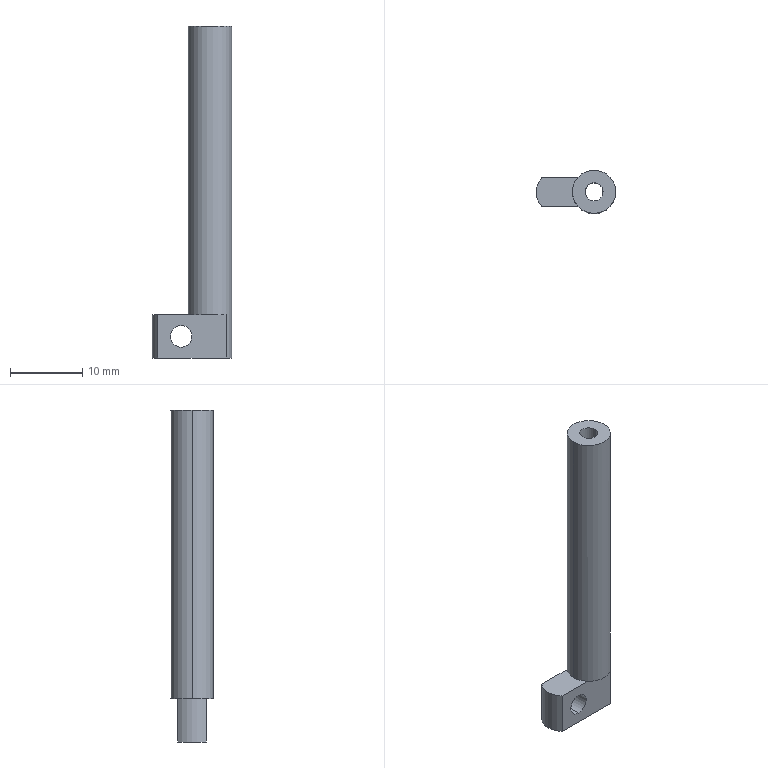Part | SolidWorks | features ICE 3, Extrusion 1 | 1 solid | 14 faces | box 11 x 6 x 46 mm | volume 1129 mm3 | cylinder 7 | plane 7 | commonest cylinder face diameters 6 x3 2.5 x2 3 x2
STEP:
#1=CARTESIAN_POINT('',(-4.,2.,-4.5));
#2=VERTEX_POINT('',#1);
#3=CARTESIAN_POINT('',(-4.,2.,-1.5));
#4=VERTEX_POINT('',#3);
#5=CARTESIAN_POINT('',(-4.,2.,-3.));
#6=DIRECTION('',(0.,1.,0.));
#7=DIRECTION('',(0.,0.,1.));
#8=AXIS2_PLACEMENT_3D('',#5,#6,#7);
#9=CIRCLE('',#8,1.5);
#10=EDGE_CURVE('',#2,#4,#9,.T.);
#11=ORIENTED_EDGE('',*,*,#10,.T.);
#12=CARTESIAN_POINT('',(-4.,-2.,-1.5));
#13=VERTEX_POINT('',#12);
#14=CARTESIAN_POINT('',(-4.,14.,-1.5));
#15=DIRECTION('',(0.,-1.,0.));
#16=VECTOR('',#15,1000.);
#17=LINE('',#14,#16);
#18=EDGE_CURVE('',#4,#13,#17,.T.);
#19=ORIENTED_EDGE('',*,*,#18,.T.);
#20=CARTESIAN_POINT('',(-4.,-2.,-4.5));
#21=VERTEX_POINT('',#20);
#22=CARTESIAN_POINT('',(-4.,-2.,-3.));
#23=DIRECTION('',(0.,-1.,0.));
#24=DIRECTION('',(0.,0.,-1.));
#25=AXIS2_PLACEMENT_3D('',#22,#23,#24);
#26=CIRCLE('',#25,1.5);
#27=EDGE_CURVE('',#13,#21,#26,.T.);
#28=ORIENTED_EDGE('',*,*,#27,.T.);
#29=CARTESIAN_POINT('',(-4.,14.,-4.5));
#30=DIRECTION('',(0.,-1.,0.));
#31=VECTOR('',#30,1000.);
#32=LINE('',#29,#31);
#33=EDGE_CURVE('',#2,#21,#32,.T.);
#34=ORIENTED_EDGE('',*,*,#33,.F.);
#35=EDGE_LOOP('',(#11,#19,#28,#34));
#36=FACE_OUTER_BOUND('',#35,.T.);
#37=CARTESIAN_POINT('',(-4.,14.,-3.));
#38=DIRECTION('',(0.,-1.,0.));
#39=DIRECTION('',(0.,0.,-1.));
#40=AXIS2_PLACEMENT_3D('',#37,#38,#39);
#41=CYLINDRICAL_SURFACE('',#40,1.5);
#42=ADVANCED_FACE('',(#36),#41,.F.);
#43=CARTESIAN_POINT('',(-1.25,0.,40.));
#44=VERTEX_POINT('',#43);
#45=CARTESIAN_POINT('',(1.25,0.,40.));
#46=VERTEX_POINT('',#45);
#47=CARTESIAN_POINT('',(0.,0.,40.));
#48=DIRECTION('',(0.,0.,1.));
#49=DIRECTION('',(1.,0.,0.));
#50=AXIS2_PLACEMENT_3D('',#47,#48,#49);
#51=CIRCLE('',#50,1.25);
#52=EDGE_CURVE('',#44,#46,#51,.T.);
#53=ORIENTED_EDGE('',*,*,#52,.T.);
#54=CARTESIAN_POINT('',(1.25,0.,-6.));
#55=VERTEX_POINT('',#54);
#56=CARTESIAN_POINT('',(1.25,0.,40.));
#57=DIRECTION('',(0.,0.,-1.));
#58=VECTOR('',#57,1000.);
#59=LINE('',#56,#58);
#60=EDGE_CURVE('',#46,#55,#59,.T.);
#61=ORIENTED_EDGE('',*,*,#60,.T.);
#62=CARTESIAN_POINT('',(-1.25,0.,-6.));
#63=VERTEX_POINT('',#62);
#64=CARTESIAN_POINT('',(0.,0.,-6.));
#65=DIRECTION('',(0.,0.,-1.));
#66=DIRECTION('',(-1.,0.,0.));
#67=AXIS2_PLACEMENT_3D('',#64,#65,#66);
#68=CIRCLE('',#67,1.25);
#69=EDGE_CURVE('',#55,#63,#68,.T.);
#70=ORIENTED_EDGE('',*,*,#69,.T.);
#71=CARTESIAN_POINT('',(-1.25,0.,40.));
#72=DIRECTION('',(0.,0.,-1.));
#73=VECTOR('',#72,1000.);
#74=LINE('',#71,#73);
#75=EDGE_CURVE('',#44,#63,#74,.T.);
#76=ORIENTED_EDGE('',*,*,#75,.F.);
#77=EDGE_LOOP('',(#53,#61,#70,#76));
#78=FACE_OUTER_BOUND('',#77,.T.);
#79=CARTESIAN_POINT('',(0.,0.,40.));
#80=DIRECTION('',(0.,0.,-1.));
#81=DIRECTION('',(-1.,0.,0.));
#82=AXIS2_PLACEMENT_3D('',#79,#80,#81);
#83=CYLINDRICAL_SURFACE('',#82,1.25);
#84=ADVANCED_FACE('',(#78),#83,.F.);
#85=CARTESIAN_POINT('',(3.,0.,40.));
#86=VERTEX_POINT('',#85);
#87=CARTESIAN_POINT('',(-3.,0.,40.));
#88=VERTEX_POINT('',#87);
#89=CARTESIAN_POINT('',(0.,0.,40.));
#90=DIRECTION('',(0.,0.,1.));
#91=DIRECTION('',(1.,0.,0.));
#92=AXIS2_PLACEMENT_3D('',#89,#90,#91);
#93=CIRCLE('',#92,3.);
#94=EDGE_CURVE('',#86,#88,#93,.T.);
#95=ORIENTED_EDGE('',*,*,#94,.F.);
#96=CARTESIAN_POINT('',(3.,0.,-6.));
#97=VERTEX_POINT('',#96);
#98=CARTESIAN_POINT('',(3.,0.,40.));
#99=DIRECTION('',(0.,0.,-1.));
#100=VECTOR('',#99,1000.);
#101=LINE('',#98,#100);
#102=EDGE_CURVE('',#86,#97,#101,.T.);
#103=ORIENTED_EDGE('',*,*,#102,.T.);
#104=CARTESIAN_POINT('',(2.236,2.,-6.));
#105=VERTEX_POINT('',#104);
#106=CARTESIAN_POINT('',(0.,0.,-6.));
#107=DIRECTION('',(0.,0.,-1.));
#108=DIRECTION('',(-1.,0.,0.));
#109=AXIS2_PLACEMENT_3D('',#106,#107,#108);
#110=CIRCLE('',#109,3.);
#111=EDGE_CURVE('',#105,#97,#110,.T.);
#112=ORIENTED_EDGE('',*,*,#111,.F.);
#113=CARTESIAN_POINT('',(2.236,2.,0.));
#114=VERTEX_POINT('',#113);
#115=CARTESIAN_POINT('',(2.236,2.,40.));
#116=DIRECTION('',(0.,0.,-1.));
#117=VECTOR('',#116,1000.);
#118=LINE('',#115,#117);
#119=EDGE_CURVE('',#114,#105,#118,.T.);
#120=ORIENTED_EDGE('',*,*,#119,.F.);
#121=CARTESIAN_POINT('',(-2.236,2.,0.));
#122=VERTEX_POINT('',#121);
#123=CARTESIAN_POINT('',(0.,0.,0.));
#124=DIRECTION('',(0.,0.,1.));
#125=DIRECTION('',(1.,0.,0.));
#126=AXIS2_PLACEMENT_3D('',#123,#124,#125);
#127=CIRCLE('',#126,3.);
#128=EDGE_CURVE('',#114,#122,#127,.T.);
#129=ORIENTED_EDGE('',*,*,#128,.T.);
#130=CARTESIAN_POINT('',(-3.,0.,0.));
#131=VERTEX_POINT('',#130);
#132=CARTESIAN_POINT('',(0.,0.,0.));
#133=DIRECTION('',(0.,0.,1.));
#134=DIRECTION('',(1.,0.,0.));
#135=AXIS2_PLACEMENT_3D('',#132,#133,#134);
#136=CIRCLE('',#135,3.);
#137=EDGE_CURVE('',#122,#131,#136,.T.);
#138=ORIENTED_EDGE('',*,*,#137,.T.);
#139=CARTESIAN_POINT('',(-3.,0.,40.));
#140=DIRECTION('',(0.,0.,-1.));
#141=VECTOR('',#140,1000.);
#142=LINE('',#139,#141);
#143=EDGE_CURVE('',#88,#131,#142,.T.);
#144=ORIENTED_EDGE('',*,*,#143,.F.);
#145=EDGE_LOOP('',(#95,#103,#112,#120,#129,#138,#144));
#146=FACE_OUTER_BOUND('',#145,.T.);
#147=CARTESIAN_POINT('',(0.,0.,40.));
#148=DIRECTION('',(0.,0.,-1.));
#149=DIRECTION('',(-1.,0.,0.));
#150=AXIS2_PLACEMENT_3D('',#147,#148,#149);
#151=CYLINDRICAL_SURFACE('',#150,3.);
#152=ADVANCED_FACE('',(#146),#151,.T.);
#153=ORIENTED_EDGE('',*,*,#102,.F.);
#154=CARTESIAN_POINT('',(0.,0.,40.));
#155=DIRECTION('',(0.,0.,1.));
#156=DIRECTION('',(1.,0.,0.));
#157=AXIS2_PLACEMENT_3D('',#154,#155,#156);
#158=CIRCLE('',#157,3.);
#159=EDGE_CURVE('',#88,#86,#158,.T.);
#160=ORIENTED_EDGE('',*,*,#159,.F.);
#161=ORIENTED_EDGE('',*,*,#143,.T.);
#162=CARTESIAN_POINT('',(-2.236,-2.,0.));
#163=VERTEX_POINT('',#162);
#164=CARTESIAN_POINT('',(0.,0.,0.));
#165=DIRECTION('',(0.,0.,1.));
#166=DIRECTION('',(1.,0.,0.));
#167=AXIS2_PLACEMENT_3D('',#164,#165,#166);
#168=CIRCLE('',#167,3.);
#169=EDGE_CURVE('',#131,#163,#168,.T.);
#170=ORIENTED_EDGE('',*,*,#169,.T.);
#171=CARTESIAN_POINT('',(2.236,-2.,0.));
#172=VERTEX_POINT('',#171);
#173=CARTESIAN_POINT('',(0.,0.,0.));
#174=DIRECTION('',(0.,0.,-1.));
#175=DIRECTION('',(-1.,0.,0.));
#176=AXIS2_PLACEMENT_3D('',#173,#174,#175);
#177=CIRCLE('',#176,3.);
#178=EDGE_CURVE('',#172,#163,#177,.T.);
#179=ORIENTED_EDGE('',*,*,#178,.F.);
#180=CARTESIAN_POINT('',(2.236,-2.,-6.));
#181=VERTEX_POINT('',#180);
#182=CARTESIAN_POINT('',(2.236,-2.,40.));
#183=DIRECTION('',(0.,0.,1.));
#184=VECTOR('',#183,1000.);
#185=LINE('',#182,#184);
#186=EDGE_CURVE('',#181,#172,#185,.T.);
#187=ORIENTED_EDGE('',*,*,#186,.F.);
#188=CARTESIAN_POINT('',(0.,0.,-6.));
#189=DIRECTION('',(0.,0.,-1.));
#190=DIRECTION('',(-1.,0.,0.));
#191=AXIS2_PLACEMENT_3D('',#188,#189,#190);
#192=CIRCLE('',#191,3.);
#193=EDGE_CURVE('',#97,#181,#192,.T.);
#194=ORIENTED_EDGE('',*,*,#193,.F.);
#195=EDGE_LOOP('',(#153,#160,#161,#170,#179,#187,#194));
#196=FACE_OUTER_BOUND('',#195,.T.);
#197=CARTESIAN_POINT('',(0.,0.,40.));
#198=DIRECTION('',(0.,0.,-1.));
#199=DIRECTION('',(-1.,0.,0.));
#200=AXIS2_PLACEMENT_3D('',#197,#198,#199);
#201=CYLINDRICAL_SURFACE('',#200,3.);
#202=ADVANCED_FACE('',(#196),#201,.T.);
#203=CARTESIAN_POINT('',(0.,0.,-6.));
#204=DIRECTION('',(0.,0.,-1.));
#205=DIRECTION('',(-1.,0.,0.));
#206=AXIS2_PLACEMENT_3D('',#203,#204,#205);
#207=CIRCLE('',#206,1.25);
#208=EDGE_CURVE('',#63,#55,#207,.T.);
#209=ORIENTED_EDGE('',*,*,#208,.F.);
#210=ORIENTED_EDGE('',*,*,#69,.F.);
#211=EDGE_LOOP('',(#209,#210));
#212=FACE_BOUND('',#211,.T.);
#213=ORIENTED_EDGE('',*,*,#111,.T.);
#214=ORIENTED_EDGE('',*,*,#193,.T.);
#215=CARTESIAN_POINT('',(-7.236,-2.,-6.));
#216=VERTEX_POINT('',#215);
#217=CARTESIAN_POINT('',(6.813,-2.,-6.));
#218=DIRECTION('',(-1.,0.,0.));
#219=VECTOR('',#218,1000.);
#220=LINE('',#217,#219);
#221=EDGE_CURVE('',#181,#216,#220,.T.);
#222=ORIENTED_EDGE('',*,*,#221,.T.);
#223=CARTESIAN_POINT('',(-7.236,2.,-6.));
#224=VERTEX_POINT('',#223);
#225=CARTESIAN_POINT('',(-5.,0.,-6.));
#226=DIRECTION('',(0.,0.,-1.));
#227=DIRECTION('',(-1.,0.,0.));
#228=AXIS2_PLACEMENT_3D('',#225,#226,#227);
#229=CIRCLE('',#228,3.);
#230=EDGE_CURVE('',#216,#224,#229,.T.);
#231=ORIENTED_EDGE('',*,*,#230,.T.);
#232=CARTESIAN_POINT('',(6.813,2.,-6.));
#233=DIRECTION('',(1.,0.,0.));
#234=VECTOR('',#233,1000.);
#235=LINE('',#232,#234);
#236=EDGE_CURVE('',#224,#105,#235,.T.);
#237=ORIENTED_EDGE('',*,*,#236,.T.);
#238=EDGE_LOOP('',(#213,#214,#222,#231,#237));
#239=FACE_OUTER_BOUND('',#238,.T.);
#240=CARTESIAN_POINT('',(0.,0.,-6.));
#241=DIRECTION('',(0.,0.,-1.));
#242=DIRECTION('',(-1.,0.,0.));
#243=AXIS2_PLACEMENT_3D('',#240,#241,#242);
#244=PLANE('',#243);
#245=ADVANCED_FACE('',(#212,#239),#244,.T.);
#246=CARTESIAN_POINT('',(-7.236,-2.,0.));
#247=VERTEX_POINT('',#246);
#248=CARTESIAN_POINT('',(6.813,-2.,0.));
#249=DIRECTION('',(-1.,0.,0.));
#250=VECTOR('',#249,1000.);
#251=LINE('',#248,#250);
#252=EDGE_CURVE('',#163,#247,#251,.T.);
#253=ORIENTED_EDGE('',*,*,#252,.F.);
#254=ORIENTED_EDGE('',*,*,#169,.F.);
#255=ORIENTED_EDGE('',*,*,#137,.F.);
#256=CARTESIAN_POINT('',(-7.236,2.,0.));
#257=VERTEX_POINT('',#256);
#258=CARTESIAN_POINT('',(6.813,2.,0.));
#259=DIRECTION('',(1.,0.,0.));
#260=VECTOR('',#259,1000.);
#261=LINE('',#258,#260);
#262=EDGE_CURVE('',#257,#122,#261,.T.);
#263=ORIENTED_EDGE('',*,*,#262,.F.);
#264=CARTESIAN_POINT('',(-5.,0.,0.));
#265=DIRECTION('',(0.,0.,-1.));
#266=DIRECTION('',(-1.,0.,0.));
#267=AXIS2_PLACEMENT_3D('',#264,#265,#266);
#268=CIRCLE('',#267,3.);
#269=EDGE_CURVE('',#247,#257,#268,.T.);
#270=ORIENTED_EDGE('',*,*,#269,.F.);
#271=EDGE_LOOP('',(#253,#254,#255,#263,#270));
#272=FACE_OUTER_BOUND('',#271,.T.);
#273=CARTESIAN_POINT('',(0.,0.,0.));
#274=DIRECTION('',(0.,0.,-1.));
#275=DIRECTION('',(-1.,0.,0.));
#276=AXIS2_PLACEMENT_3D('',#273,#274,#275);
#277=PLANE('',#276);
#278=ADVANCED_FACE('',(#272),#277,.F.);
#279=CARTESIAN_POINT('',(-7.236,-2.,-6.));
#280=DIRECTION('',(0.,0.,-1.));
#281=VECTOR('',#280,1000.);
#282=LINE('',#279,#281);
#283=EDGE_CURVE('',#247,#216,#282,.T.);
#284=ORIENTED_EDGE('',*,*,#283,.F.);
#285=ORIENTED_EDGE('',*,*,#269,.T.);
#286=CARTESIAN_POINT('',(-7.236,2.,-6.));
#287=DIRECTION('',(0.,0.,1.));
#288=VECTOR('',#287,1000.);
#289=LINE('',#286,#288);
#290=EDGE_CURVE('',#224,#257,#289,.T.);
#291=ORIENTED_EDGE('',*,*,#290,.F.);
#292=ORIENTED_EDGE('',*,*,#230,.F.);
#293=EDGE_LOOP('',(#284,#285,#291,#292));
#294=FACE_OUTER_BOUND('',#293,.T.);
#295=CARTESIAN_POINT('',(-5.,0.,-6.));
#296=DIRECTION('',(0.,0.,1.));
#297=DIRECTION('',(1.,0.,0.));
#298=AXIS2_PLACEMENT_3D('',#295,#296,#297);
#299=CYLINDRICAL_SURFACE('',#298,3.);
#300=ADVANCED_FACE('',(#294),#299,.T.);
#301=ORIENTED_EDGE('',*,*,#159,.T.);
#302=ORIENTED_EDGE('',*,*,#94,.T.);
#303=EDGE_LOOP('',(#301,#302));
#304=FACE_OUTER_BOUND('',#303,.T.);
#305=ORIENTED_EDGE('',*,*,#52,.F.);
#306=CARTESIAN_POINT('',(0.,0.,40.));
#307=DIRECTION('',(0.,0.,1.));
#308=DIRECTION('',(1.,0.,0.));
#309=AXIS2_PLACEMENT_3D('',#306,#307,#308);
#310=CIRCLE('',#309,1.25);
#311=EDGE_CURVE('',#46,#44,#310,.T.);
#312=ORIENTED_EDGE('',*,*,#311,.F.);
#313=EDGE_LOOP('',(#305,#312));
#314=FACE_BOUND('',#313,.T.);
#315=CARTESIAN_POINT('',(0.,0.,40.));
#316=DIRECTION('',(0.,0.,1.));
#317=DIRECTION('',(1.,0.,0.));
#318=AXIS2_PLACEMENT_3D('',#315,#316,#317);
#319=PLANE('',#318);
#320=ADVANCED_FACE('',(#304,#314),#319,.T.);
#321=ORIENTED_EDGE('',*,*,#60,.F.);
#322=ORIENTED_EDGE('',*,*,#311,.T.);
#323=ORIENTED_EDGE('',*,*,#75,.T.);
#324=ORIENTED_EDGE('',*,*,#208,.T.);
#325=EDGE_LOOP('',(#321,#322,#323,#324));
#326=FACE_OUTER_BOUND('',#325,.T.);
#327=CARTESIAN_POINT('',(0.,0.,40.));
#328=DIRECTION('',(0.,0.,-1.));
#329=DIRECTION('',(-1.,0.,0.));
#330=AXIS2_PLACEMENT_3D('',#327,#328,#329);
#331=CYLINDRICAL_SURFACE('',#330,1.25);
#332=ADVANCED_FACE('',(#326),#331,.F.);
#333=ORIENTED_EDGE('',*,*,#10,.F.);
#334=CARTESIAN_POINT('',(-4.,2.,-3.));
#335=DIRECTION('',(0.,1.,0.));
#336=DIRECTION('',(0.,0.,1.));
#337=AXIS2_PLACEMENT_3D('',#334,#335,#336);
#338=CIRCLE('',#337,1.5);
#339=EDGE_CURVE('',#4,#2,#338,.T.);
#340=ORIENTED_EDGE('',*,*,#339,.F.);
#341=EDGE_LOOP('',(#333,#340));
#342=FACE_BOUND('',#341,.T.);
#343=ORIENTED_EDGE('',*,*,#119,.T.);
#344=ORIENTED_EDGE('',*,*,#236,.F.);
#345=ORIENTED_EDGE('',*,*,#290,.T.);
#346=ORIENTED_EDGE('',*,*,#262,.T.);
#347=CARTESIAN_POINT('',(6.813,2.,0.));
#348=DIRECTION('',(1.,0.,0.));
#349=VECTOR('',#348,1000.);
#350=LINE('',#347,#349);
#351=EDGE_CURVE('',#122,#114,#350,.T.);
#352=ORIENTED_EDGE('',*,*,#351,.T.);
#353=EDGE_LOOP('',(#343,#344,#345,#346,#352));
#354=FACE_OUTER_BOUND('',#353,.T.);
#355=CARTESIAN_POINT('',(6.813,2.,0.));
#356=DIRECTION('',(0.,1.,0.));
#357=DIRECTION('',(0.,0.,1.));
#358=AXIS2_PLACEMENT_3D('',#355,#356,#357);
#359=PLANE('',#358);
#360=ADVANCED_FACE('',(#342,#354),#359,.T.);
#361=ORIENTED_EDGE('',*,*,#128,.F.);
#362=ORIENTED_EDGE('',*,*,#351,.F.);
#363=EDGE_LOOP('',(#361,#362));
#364=FACE_OUTER_BOUND('',#363,.T.);
#365=CARTESIAN_POINT('',(0.,0.,0.));
#366=DIRECTION('',(0.,0.,-1.));
#367=DIRECTION('',(-1.,0.,0.));
#368=AXIS2_PLACEMENT_3D('',#365,#366,#367);
#369=PLANE('',#368);
#370=ADVANCED_FACE('',(#364),#369,.T.);
#371=CARTESIAN_POINT('',(-4.,-2.,-3.));
#372=DIRECTION('',(0.,-1.,0.));
#373=DIRECTION('',(0.,0.,-1.));
#374=AXIS2_PLACEMENT_3D('',#371,#372,#373);
#375=CIRCLE('',#374,1.5);
#376=EDGE_CURVE('',#21,#13,#375,.T.);
#377=ORIENTED_EDGE('',*,*,#376,.F.);
#378=ORIENTED_EDGE('',*,*,#27,.F.);
#379=EDGE_LOOP('',(#377,#378));
#380=FACE_BOUND('',#379,.T.);
#381=ORIENTED_EDGE('',*,*,#186,.T.);
#382=CARTESIAN_POINT('',(6.813,-2.,0.));
#383=DIRECTION('',(-1.,0.,0.));
#384=VECTOR('',#383,1000.);
#385=LINE('',#382,#384);
#386=EDGE_CURVE('',#172,#163,#385,.T.);
#387=ORIENTED_EDGE('',*,*,#386,.T.);
#388=ORIENTED_EDGE('',*,*,#252,.T.);
#389=ORIENTED_EDGE('',*,*,#283,.T.);
#390=ORIENTED_EDGE('',*,*,#221,.F.);
#391=EDGE_LOOP('',(#381,#387,#388,#389,#390));
#392=FACE_OUTER_BOUND('',#391,.T.);
#393=CARTESIAN_POINT('',(6.813,-2.,0.));
#394=DIRECTION('',(0.,-1.,0.));
#395=DIRECTION('',(0.,0.,-1.));
#396=AXIS2_PLACEMENT_3D('',#393,#394,#395);
#397=PLANE('',#396);
#398=ADVANCED_FACE('',(#380,#392),#397,.T.);
#399=ORIENTED_EDGE('',*,*,#178,.T.);
#400=ORIENTED_EDGE('',*,*,#386,.F.);
#401=EDGE_LOOP('',(#399,#400));
#402=FACE_OUTER_BOUND('',#401,.T.);
#403=CARTESIAN_POINT('',(0.,0.,0.));
#404=DIRECTION('',(0.,0.,-1.));
#405=DIRECTION('',(-1.,0.,0.));
#406=AXIS2_PLACEMENT_3D('',#403,#404,#405);
#407=PLANE('',#406);
#408=ADVANCED_FACE('',(#402),#407,.T.);
#409=ORIENTED_EDGE('',*,*,#18,.F.);
#410=ORIENTED_EDGE('',*,*,#339,.T.);
#411=ORIENTED_EDGE('',*,*,#33,.T.);
#412=ORIENTED_EDGE('',*,*,#376,.T.);
#413=EDGE_LOOP('',(#409,#410,#411,#412));
#414=FACE_OUTER_BOUND('',#413,.T.);
#415=CARTESIAN_POINT('',(-4.,14.,-3.));
#416=DIRECTION('',(0.,-1.,0.));
#417=DIRECTION('',(0.,0.,-1.));
#418=AXIS2_PLACEMENT_3D('',#415,#416,#417);
#419=CYLINDRICAL_SURFACE('',#418,1.5);
#420=ADVANCED_FACE('',(#414),#419,.F.);
#421=CLOSED_SHELL('',(#42,#84,#152,#202,#245,#278,#300,#320,#332,#360,#370,#398,#408,#420));
#422=MANIFOLD_SOLID_BREP('',#421);
#423=CARTESIAN_POINT('',(0.,0.,0.));
#424=DIRECTION('',(0.,0.,1.));
#425=DIRECTION('',(1.,0.,0.));
#426=AXIS2_PLACEMENT_3D('',#423,#424,#425);
#427=(LENGTH_UNIT()NAMED_UNIT(*)SI_UNIT(.MILLI.,.METRE.));
#428=UNCERTAINTY_MEASURE_WITH_UNIT(LENGTH_MEASURE(0.00001),#427,'','');
#429=(NAMED_UNIT(*)PLANE_ANGLE_UNIT()SI_UNIT($,.RADIAN.));
#430=(NAMED_UNIT(*)SI_UNIT($,.STERADIAN.)SOLID_ANGLE_UNIT());
#431=(GEOMETRIC_REPRESENTATION_CONTEXT(3)GLOBAL_UNCERTAINTY_ASSIGNED_CONTEXT((#428))GLOBAL_UNIT_ASSIGNED_CONTEXT((#427,#429,#430))REPRESENTATION_CONTEXT('',''));
#432=ADVANCED_BREP_SHAPE_REPRESENTATION('',(#422,#426),#431);